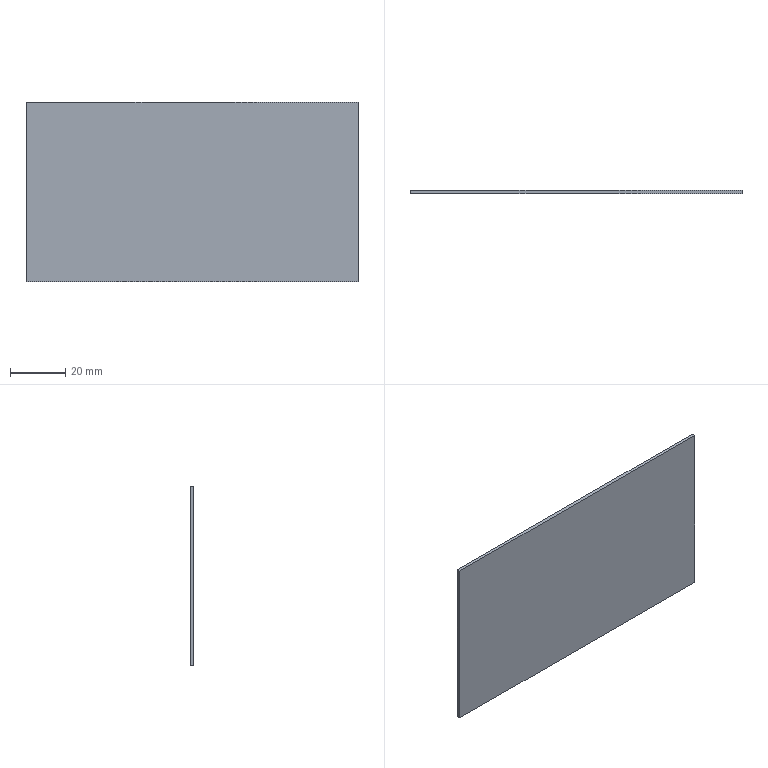Part | STEP file | JBJ-P-1003-07 | 1 solid | 6 faces | box 120 x 1.2 x 65 mm | volume 9360 mm3 | plane 6
STEP:
#1=CARTESIAN_POINT('',(0.,0.,0.));
#2=VERTEX_POINT('',#1);
#3=CARTESIAN_POINT('',(0.,0.,65.));
#4=VERTEX_POINT('',#3);
#5=CARTESIAN_POINT('',(0.,0.,0.));
#6=DIRECTION('',(0.,0.,1.));
#7=VECTOR('',#6,1000.);
#8=LINE('',#5,#7);
#9=EDGE_CURVE('',#2,#4,#8,.T.);
#10=ORIENTED_EDGE('',*,*,#9,.T.);
#11=CARTESIAN_POINT('',(0.,1.2,65.));
#12=VERTEX_POINT('',#11);
#13=CARTESIAN_POINT('',(0.,1.2,65.));
#14=DIRECTION('',(0.,-1.,0.));
#15=VECTOR('',#14,1000.);
#16=LINE('',#13,#15);
#17=EDGE_CURVE('',#12,#4,#16,.T.);
#18=ORIENTED_EDGE('',*,*,#17,.F.);
#19=CARTESIAN_POINT('',(0.,1.2,0.));
#20=VERTEX_POINT('',#19);
#21=CARTESIAN_POINT('',(0.,1.2,0.));
#22=DIRECTION('',(0.,0.,1.));
#23=VECTOR('',#22,1000.);
#24=LINE('',#21,#23);
#25=EDGE_CURVE('',#20,#12,#24,.T.);
#26=ORIENTED_EDGE('',*,*,#25,.F.);
#27=CARTESIAN_POINT('',(0.,1.2,0.));
#28=DIRECTION('',(0.,-1.,0.));
#29=VECTOR('',#28,1000.);
#30=LINE('',#27,#29);
#31=EDGE_CURVE('',#20,#2,#30,.T.);
#32=ORIENTED_EDGE('',*,*,#31,.T.);
#33=EDGE_LOOP('',(#10,#18,#26,#32));
#34=FACE_OUTER_BOUND('',#33,.T.);
#35=CARTESIAN_POINT('',(0.,1.2,0.));
#36=DIRECTION('',(1.,0.,0.));
#37=DIRECTION('',(0.,0.,-1.));
#38=AXIS2_PLACEMENT_3D('',#35,#36,#37);
#39=PLANE('',#38);
#40=ADVANCED_FACE('',(#34),#39,.F.);
#41=CARTESIAN_POINT('',(120.,0.,65.));
#42=VERTEX_POINT('',#41);
#43=CARTESIAN_POINT('',(0.,0.,65.));
#44=DIRECTION('',(1.,0.,0.));
#45=VECTOR('',#44,1000.);
#46=LINE('',#43,#45);
#47=EDGE_CURVE('',#4,#42,#46,.T.);
#48=ORIENTED_EDGE('',*,*,#47,.T.);
#49=CARTESIAN_POINT('',(120.,1.2,65.));
#50=VERTEX_POINT('',#49);
#51=CARTESIAN_POINT('',(120.,1.2,65.));
#52=DIRECTION('',(0.,-1.,0.));
#53=VECTOR('',#52,1000.);
#54=LINE('',#51,#53);
#55=EDGE_CURVE('',#50,#42,#54,.T.);
#56=ORIENTED_EDGE('',*,*,#55,.F.);
#57=CARTESIAN_POINT('',(0.,1.2,65.));
#58=DIRECTION('',(1.,0.,0.));
#59=VECTOR('',#58,1000.);
#60=LINE('',#57,#59);
#61=EDGE_CURVE('',#12,#50,#60,.T.);
#62=ORIENTED_EDGE('',*,*,#61,.F.);
#63=ORIENTED_EDGE('',*,*,#17,.T.);
#64=EDGE_LOOP('',(#48,#56,#62,#63));
#65=FACE_OUTER_BOUND('',#64,.T.);
#66=CARTESIAN_POINT('',(0.,1.2,65.));
#67=DIRECTION('',(0.,0.,-1.));
#68=DIRECTION('',(-1.,0.,0.));
#69=AXIS2_PLACEMENT_3D('',#66,#67,#68);
#70=PLANE('',#69);
#71=ADVANCED_FACE('',(#65),#70,.F.);
#72=CARTESIAN_POINT('',(120.,0.,0.));
#73=VERTEX_POINT('',#72);
#74=CARTESIAN_POINT('',(120.,0.,0.));
#75=DIRECTION('',(0.,0.,-1.));
#76=VECTOR('',#75,1000.);
#77=LINE('',#74,#76);
#78=EDGE_CURVE('',#42,#73,#77,.T.);
#79=ORIENTED_EDGE('',*,*,#78,.T.);
#80=CARTESIAN_POINT('',(120.,1.2,0.));
#81=VERTEX_POINT('',#80);
#82=CARTESIAN_POINT('',(120.,1.2,0.));
#83=DIRECTION('',(0.,-1.,0.));
#84=VECTOR('',#83,1000.);
#85=LINE('',#82,#84);
#86=EDGE_CURVE('',#81,#73,#85,.T.);
#87=ORIENTED_EDGE('',*,*,#86,.F.);
#88=CARTESIAN_POINT('',(120.,1.2,0.));
#89=DIRECTION('',(0.,0.,-1.));
#90=VECTOR('',#89,1000.);
#91=LINE('',#88,#90);
#92=EDGE_CURVE('',#50,#81,#91,.T.);
#93=ORIENTED_EDGE('',*,*,#92,.F.);
#94=ORIENTED_EDGE('',*,*,#55,.T.);
#95=EDGE_LOOP('',(#79,#87,#93,#94));
#96=FACE_OUTER_BOUND('',#95,.T.);
#97=CARTESIAN_POINT('',(120.,1.2,0.));
#98=DIRECTION('',(-1.,0.,0.));
#99=DIRECTION('',(0.,0.,1.));
#100=AXIS2_PLACEMENT_3D('',#97,#98,#99);
#101=PLANE('',#100);
#102=ADVANCED_FACE('',(#96),#101,.F.);
#103=CARTESIAN_POINT('',(0.,0.,0.));
#104=DIRECTION('',(-1.,0.,0.));
#105=VECTOR('',#104,1000.);
#106=LINE('',#103,#105);
#107=EDGE_CURVE('',#73,#2,#106,.T.);
#108=ORIENTED_EDGE('',*,*,#107,.T.);
#109=ORIENTED_EDGE('',*,*,#31,.F.);
#110=CARTESIAN_POINT('',(0.,1.2,0.));
#111=DIRECTION('',(-1.,0.,0.));
#112=VECTOR('',#111,1000.);
#113=LINE('',#110,#112);
#114=EDGE_CURVE('',#81,#20,#113,.T.);
#115=ORIENTED_EDGE('',*,*,#114,.F.);
#116=ORIENTED_EDGE('',*,*,#86,.T.);
#117=EDGE_LOOP('',(#108,#109,#115,#116));
#118=FACE_OUTER_BOUND('',#117,.T.);
#119=CARTESIAN_POINT('',(0.,1.2,0.));
#120=DIRECTION('',(0.,0.,1.));
#121=DIRECTION('',(1.,0.,0.));
#122=AXIS2_PLACEMENT_3D('',#119,#120,#121);
#123=PLANE('',#122);
#124=ADVANCED_FACE('',(#118),#123,.F.);
#125=ORIENTED_EDGE('',*,*,#25,.T.);
#126=ORIENTED_EDGE('',*,*,#61,.T.);
#127=ORIENTED_EDGE('',*,*,#92,.T.);
#128=ORIENTED_EDGE('',*,*,#114,.T.);
#129=EDGE_LOOP('',(#125,#126,#127,#128));
#130=FACE_OUTER_BOUND('',#129,.T.);
#131=CARTESIAN_POINT('',(0.,1.2,0.));
#132=DIRECTION('',(0.,1.,0.));
#133=DIRECTION('',(0.,0.,1.));
#134=AXIS2_PLACEMENT_3D('',#131,#132,#133);
#135=PLANE('',#134);
#136=ADVANCED_FACE('',(#130),#135,.T.);
#137=ORIENTED_EDGE('',*,*,#9,.F.);
#138=ORIENTED_EDGE('',*,*,#107,.F.);
#139=ORIENTED_EDGE('',*,*,#78,.F.);
#140=ORIENTED_EDGE('',*,*,#47,.F.);
#141=EDGE_LOOP('',(#137,#138,#139,#140));
#142=FACE_OUTER_BOUND('',#141,.T.);
#143=CARTESIAN_POINT('',(0.,0.,0.));
#144=DIRECTION('',(0.,1.,0.));
#145=DIRECTION('',(0.,0.,1.));
#146=AXIS2_PLACEMENT_3D('',#143,#144,#145);
#147=PLANE('',#146);
#148=ADVANCED_FACE('',(#142),#147,.F.);
#149=CLOSED_SHELL('',(#40,#71,#102,#124,#136,#148));
#150=MANIFOLD_SOLID_BREP('',#149);
#151=CARTESIAN_POINT('',(0.,0.,0.));
#152=DIRECTION('',(0.,0.,1.));
#153=DIRECTION('',(1.,0.,0.));
#154=AXIS2_PLACEMENT_3D('',#151,#152,#153);
#155=(LENGTH_UNIT()NAMED_UNIT(*)SI_UNIT(.MILLI.,.METRE.));
#156=UNCERTAINTY_MEASURE_WITH_UNIT(LENGTH_MEASURE(0.00001),#155,'','');
#157=(NAMED_UNIT(*)PLANE_ANGLE_UNIT()SI_UNIT($,.RADIAN.));
#158=(NAMED_UNIT(*)SI_UNIT($,.STERADIAN.)SOLID_ANGLE_UNIT());
#159=(GEOMETRIC_REPRESENTATION_CONTEXT(3)GLOBAL_UNCERTAINTY_ASSIGNED_CONTEXT((#156))GLOBAL_UNIT_ASSIGNED_CONTEXT((#155,#157,#158))REPRESENTATION_CONTEXT('',''));
#160=ADVANCED_BREP_SHAPE_REPRESENTATION('',(#150,#154),#159);